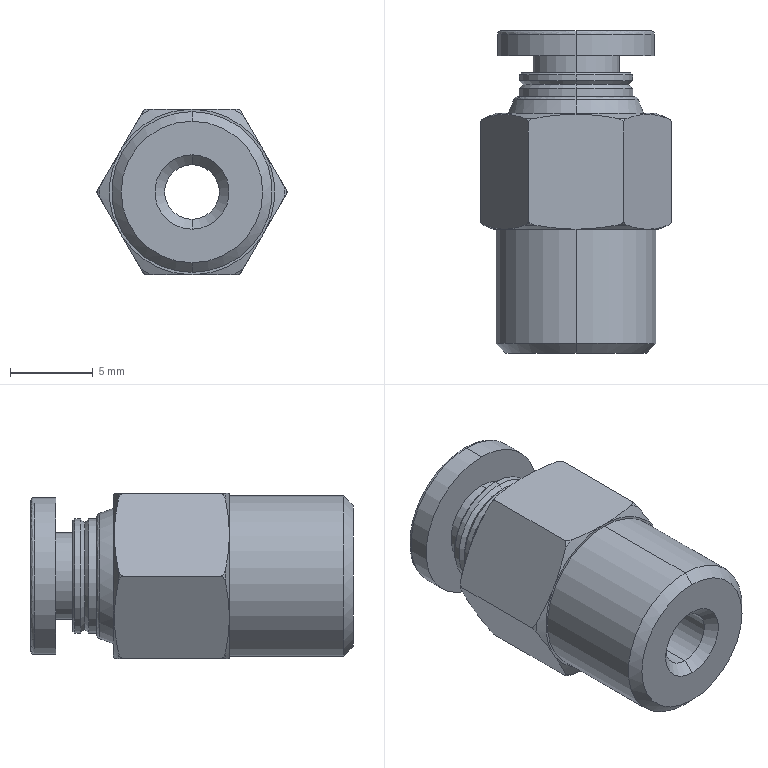Part | STEP file | 11-pc401-V2.0-V2.011 | 1 solid | 66 faces | box 11.547 x 19.5 x 10 mm | volume 1161 mm3 | cone 20 | spline 18 | cylinder 14 | plane 14 | commonest cylinder face diameters 6.9 x4 3.3 x2 4 x2 5.26 x2 9.5 x2 9.728 x2